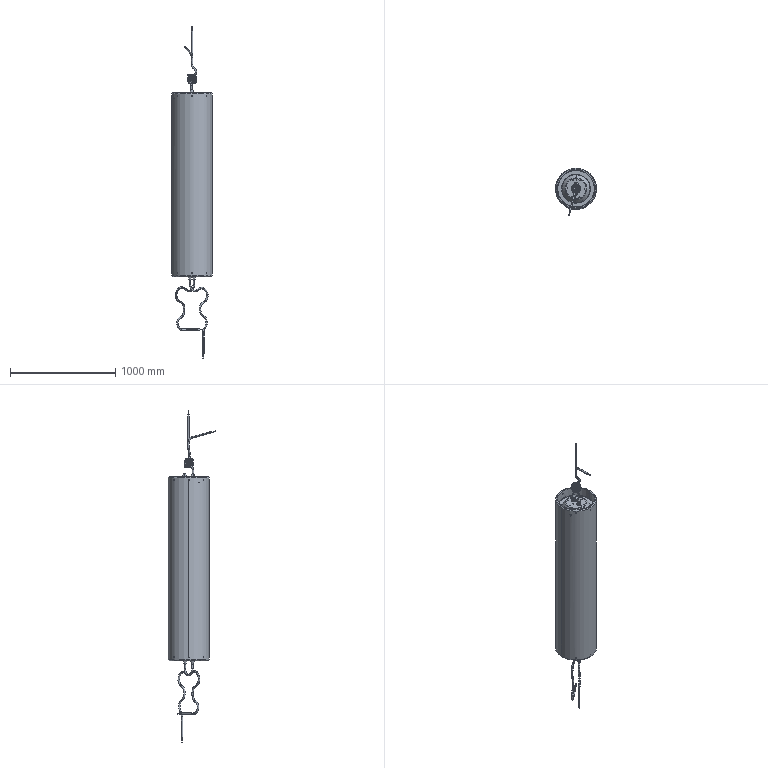Part | NX | features BREP 13 | 15 solids | 1845 faces | box 390 x 453.508 x 3159 mm | volume 86881818 mm3 | cylinder 571 | cone 451 | spline 398 | torus 210 | plane 209 | sphere 6 | commonest cylinder face diameters 30 x104 26 x96 6.35 x37 6.8 x36 4.2 x32 10.2 x32